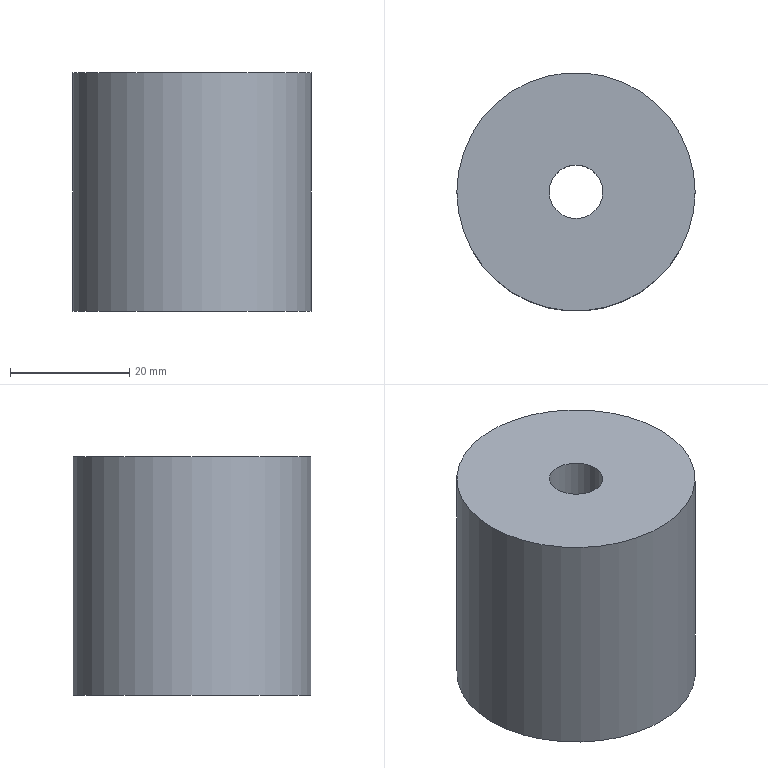Part | STEP file | gslz 2016.10.28-10_id2442_x_t | 1 solid | 6 faces | box 40 x 40 x 40 mm | volume 45553 mm3 | cylinder 3 | plane 3 | commonest cylinder face diameters 9 x1 14 x1 40 x1
STEP:
#1=CARTESIAN_POINT('',(0.,0.,0.));
#2=DIRECTION('',(0.,0.,1.));
#3=DIRECTION('',(1.,0.,0.));
#4=AXIS2_PLACEMENT_3D('',#1,#2,#3);
#5=CARTESIAN_POINT('',(-61.5,235.,105.));
#6=VERTEX_POINT('',#5);
#7=CARTESIAN_POINT('',(-81.5,235.,105.));
#8=DIRECTION('',(0.,0.,1.));
#9=DIRECTION('',(1.,0.,0.));
#10=AXIS2_PLACEMENT_3D('',#7,#8,#9);
#11=CIRCLE('',#10,20.);
#12=CARTESIAN_POINT('',(-81.5,235.,60.));
#13=DIRECTION('',(0.,0.,1.));
#14=DIRECTION('',(1.,0.,0.));
#15=AXIS2_PLACEMENT_3D('',#12,#13,#14);
#16=CYLINDRICAL_SURFACE('',#15,20.);
#17=CARTESIAN_POINT('',(0.,45.));
#18=DIRECTION('',(1.,0.));
#19=VECTOR('',#18,1.);
#20=LINE('',#17,#19);
#21=(GEOMETRIC_REPRESENTATION_CONTEXT(2)PARAMETRIC_REPRESENTATION_CONTEXT()REPRESENTATION_CONTEXT('',''));
#22=DEFINITIONAL_REPRESENTATION('',(#20),#21);
#23=PCURVE('',#16,#22);
#24=CARTESIAN_POINT('',(-29.389,-253.723,105.));
#25=DIRECTION('',(0.,0.,1.));
#26=DIRECTION('',(1.,0.,0.));
#27=AXIS2_PLACEMENT_3D('',#24,#25,#26);
#28=PLANE('',#27);
#29=CARTESIAN_POINT('',(-52.111,488.723));
#30=DIRECTION('',(1.,0.));
#31=AXIS2_PLACEMENT_2D('',#29,#30);
#32=CIRCLE('',#31,20.);
#33=(GEOMETRIC_REPRESENTATION_CONTEXT(2)PARAMETRIC_REPRESENTATION_CONTEXT()REPRESENTATION_CONTEXT('',''));
#34=DEFINITIONAL_REPRESENTATION('',(#32),#33);
#35=PCURVE('',#28,#34);
#36=SURFACE_CURVE('',#11,(#23,#35),.PCURVE_S1.);
#37=EDGE_CURVE('',#6,#6,#36,.T.);
#38=ORIENTED_EDGE('',*,*,#37,.F.);
#39=CARTESIAN_POINT('',(-61.5,235.,65.));
#40=VERTEX_POINT('',#39);
#41=CARTESIAN_POINT('',(-61.5,235.,65.));
#42=CARTESIAN_POINT('',(-61.5,235.,105.));
#43=B_SPLINE_CURVE_WITH_KNOTS('',1,(#41,#42),.UNSPECIFIED.,.F.,.F.,(2,2),(5.,45.),.PIECEWISE_BEZIER_KNOTS.);
#44=CARTESIAN_POINT('',(0.,0.));
#45=DIRECTION('',(0.,1.));
#46=VECTOR('',#45,1.);
#47=LINE('',#44,#46);
#48=(GEOMETRIC_REPRESENTATION_CONTEXT(2)PARAMETRIC_REPRESENTATION_CONTEXT()REPRESENTATION_CONTEXT('',''));
#49=DEFINITIONAL_REPRESENTATION('',(#47),#48);
#50=PCURVE('',#16,#49);
#51=CARTESIAN_POINT('',(6.283,0.));
#52=DIRECTION('',(0.,1.));
#53=VECTOR('',#52,1.);
#54=LINE('',#51,#53);
#55=(GEOMETRIC_REPRESENTATION_CONTEXT(2)PARAMETRIC_REPRESENTATION_CONTEXT()REPRESENTATION_CONTEXT('',''));
#56=DEFINITIONAL_REPRESENTATION('',(#54),#55);
#57=PCURVE('',#16,#56);
#58=SEAM_CURVE('',#43,(#50,#57),.PCURVE_S1.);
#59=EDGE_CURVE('',#40,#6,#58,.T.);
#60=ORIENTED_EDGE('',*,*,#59,.F.);
#61=CARTESIAN_POINT('',(-101.5,235.,65.));
#62=VERTEX_POINT('',#61);
#63=CARTESIAN_POINT('',(-81.5,235.,65.));
#64=DIRECTION('',(0.,0.,1.));
#65=DIRECTION('',(-1.,0.,0.));
#66=AXIS2_PLACEMENT_3D('',#63,#64,#65);
#67=CIRCLE('',#66,20.);
#68=CARTESIAN_POINT('',(-3.142,5.));
#69=DIRECTION('',(1.,0.));
#70=VECTOR('',#69,1.);
#71=LINE('',#68,#70);
#72=(GEOMETRIC_REPRESENTATION_CONTEXT(2)PARAMETRIC_REPRESENTATION_CONTEXT()REPRESENTATION_CONTEXT('',''));
#73=DEFINITIONAL_REPRESENTATION('',(#71),#72);
#74=PCURVE('',#16,#73);
#75=CARTESIAN_POINT('',(-81.5,235.,65.));
#76=DIRECTION('',(0.,0.,-1.));
#77=DIRECTION('',(-1.,0.,0.));
#78=AXIS2_PLACEMENT_3D('',#75,#76,#77);
#79=PLANE('',#78);
#80=CARTESIAN_POINT('',(20.,0.));
#81=CARTESIAN_POINT('',(20.,-34.641));
#82=CARTESIAN_POINT('',(-10.,-17.321));
#83=CARTESIAN_POINT('',(-40.,0.));
#84=CARTESIAN_POINT('',(-10.,17.321));
#85=CARTESIAN_POINT('',(20.,34.641));
#86=CARTESIAN_POINT('',(20.,0.));
#87=(BOUNDED_CURVE()B_SPLINE_CURVE(2,(#80,#81,#82,#83,#84,#85,#86),.UNSPECIFIED.,.T.,.F.)B_SPLINE_CURVE_WITH_KNOTS((1,2,2,2,2,1),(-2.094,0.,2.094,4.189,6.283,8.378),.UNSPECIFIED.)CURVE()GEOMETRIC_REPRESENTATION_ITEM()RATIONAL_B_SPLINE_CURVE((1.,0.5,1.,0.5,1.,0.5,1.))REPRESENTATION_ITEM(''));
#88=(GEOMETRIC_REPRESENTATION_CONTEXT(2)PARAMETRIC_REPRESENTATION_CONTEXT()REPRESENTATION_CONTEXT('',''));
#89=DEFINITIONAL_REPRESENTATION('',(#87),#88);
#90=PCURVE('',#79,#89);
#91=SURFACE_CURVE('',#67,(#74,#90),.PCURVE_S1.);
#92=EDGE_CURVE('',#40,#62,#91,.T.);
#93=ORIENTED_EDGE('',*,*,#92,.T.);
#94=CARTESIAN_POINT('',(-81.5,235.,65.));
#95=DIRECTION('',(0.,0.,1.));
#96=DIRECTION('',(-1.,0.,0.));
#97=AXIS2_PLACEMENT_3D('',#94,#95,#96);
#98=CIRCLE('',#97,20.);
#99=CARTESIAN_POINT('',(3.142,5.));
#100=DIRECTION('',(1.,0.));
#101=VECTOR('',#100,1.);
#102=LINE('',#99,#101);
#103=(GEOMETRIC_REPRESENTATION_CONTEXT(2)PARAMETRIC_REPRESENTATION_CONTEXT()REPRESENTATION_CONTEXT('',''));
#104=DEFINITIONAL_REPRESENTATION('',(#102),#103);
#105=PCURVE('',#16,#104);
#106=CARTESIAN_POINT('',(20.,0.));
#107=CARTESIAN_POINT('',(20.,-34.641));
#108=CARTESIAN_POINT('',(-10.,-17.321));
#109=CARTESIAN_POINT('',(-40.,0.));
#110=CARTESIAN_POINT('',(-10.,17.321));
#111=CARTESIAN_POINT('',(20.,34.641));
#112=CARTESIAN_POINT('',(20.,0.));
#113=(BOUNDED_CURVE()B_SPLINE_CURVE(2,(#106,#107,#108,#109,#110,#111,#112),.UNSPECIFIED.,.T.,.F.)B_SPLINE_CURVE_WITH_KNOTS((1,2,2,2,2,1),(-2.094,0.,2.094,4.189,6.283,8.378),.UNSPECIFIED.)CURVE()GEOMETRIC_REPRESENTATION_ITEM()RATIONAL_B_SPLINE_CURVE((1.,0.5,1.,0.5,1.,0.5,1.))REPRESENTATION_ITEM(''));
#114=(GEOMETRIC_REPRESENTATION_CONTEXT(2)PARAMETRIC_REPRESENTATION_CONTEXT()REPRESENTATION_CONTEXT('',''));
#115=DEFINITIONAL_REPRESENTATION('',(#113),#114);
#116=PCURVE('',#79,#115);
#117=SURFACE_CURVE('',#98,(#105,#116),.PCURVE_S1.);
#118=EDGE_CURVE('',#62,#40,#117,.T.);
#119=ORIENTED_EDGE('',*,*,#118,.T.);
#120=ORIENTED_EDGE('',*,*,#59,.T.);
#121=EDGE_LOOP('',(#38,#60,#93,#119,#120));
#122=FACE_BOUND('',#121,.T.);
#123=ADVANCED_FACE('',(#122),#16,.T.);
#124=CARTESIAN_POINT('',(-77.,235.,105.));
#125=VERTEX_POINT('',#124);
#126=CARTESIAN_POINT('',(-81.5,235.,105.));
#127=DIRECTION('',(0.,0.,1.));
#128=DIRECTION('',(1.,0.,0.));
#129=AXIS2_PLACEMENT_3D('',#126,#127,#128);
#130=CIRCLE('',#129,4.5);
#131=CARTESIAN_POINT('',(-52.111,488.723));
#132=DIRECTION('',(1.,0.));
#133=AXIS2_PLACEMENT_2D('',#131,#132);
#134=CIRCLE('',#133,4.5);
#135=(GEOMETRIC_REPRESENTATION_CONTEXT(2)PARAMETRIC_REPRESENTATION_CONTEXT()REPRESENTATION_CONTEXT('',''));
#136=DEFINITIONAL_REPRESENTATION('',(#134),#135);
#137=PCURVE('',#28,#136);
#138=CARTESIAN_POINT('',(-81.5,235.,37.));
#139=DIRECTION('',(0.,0.,1.));
#140=DIRECTION('',(1.,0.,0.));
#141=AXIS2_PLACEMENT_3D('',#138,#139,#140);
#142=CYLINDRICAL_SURFACE('',#141,4.5);
#143=CARTESIAN_POINT('',(0.,68.));
#144=DIRECTION('',(1.,0.));
#145=VECTOR('',#144,1.);
#146=LINE('',#143,#145);
#147=(GEOMETRIC_REPRESENTATION_CONTEXT(2)PARAMETRIC_REPRESENTATION_CONTEXT()REPRESENTATION_CONTEXT('',''));
#148=DEFINITIONAL_REPRESENTATION('',(#146),#147);
#149=PCURVE('',#142,#148);
#150=SURFACE_CURVE('',#130,(#137,#149),.PCURVE_S1.);
#151=EDGE_CURVE('',#125,#125,#150,.T.);
#152=ORIENTED_EDGE('',*,*,#151,.F.);
#153=EDGE_LOOP('',(#152));
#154=FACE_BOUND('',#153,.T.);
#155=ORIENTED_EDGE('',*,*,#37,.T.);
#156=EDGE_LOOP('',(#155));
#157=FACE_BOUND('',#156,.T.);
#158=ADVANCED_FACE('',(#154,#157),#28,.T.);
#159=ORIENTED_EDGE('',*,*,#118,.F.);
#160=ORIENTED_EDGE('',*,*,#92,.F.);
#161=EDGE_LOOP('',(#159,#160));
#162=FACE_BOUND('',#161,.T.);
#163=CARTESIAN_POINT('',(-88.5,235.,65.));
#164=VERTEX_POINT('',#163);
#165=CARTESIAN_POINT('',(-81.5,235.,65.));
#166=DIRECTION('',(0.,0.,1.));
#167=DIRECTION('',(-1.,0.,0.));
#168=AXIS2_PLACEMENT_3D('',#165,#166,#167);
#169=CIRCLE('',#168,7.);
#170=CARTESIAN_POINT('',(7.,0.));
#171=CARTESIAN_POINT('',(7.,-12.124));
#172=CARTESIAN_POINT('',(-3.5,-6.062));
#173=CARTESIAN_POINT('',(-14.,0.));
#174=CARTESIAN_POINT('',(-3.5,6.062));
#175=CARTESIAN_POINT('',(7.,12.124));
#176=CARTESIAN_POINT('',(7.,0.));
#177=(BOUNDED_CURVE()B_SPLINE_CURVE(2,(#170,#171,#172,#173,#174,#175,#176),.UNSPECIFIED.,.T.,.F.)B_SPLINE_CURVE_WITH_KNOTS((1,2,2,2,2,1),(-2.094,0.,2.094,4.189,6.283,8.378),.UNSPECIFIED.)CURVE()GEOMETRIC_REPRESENTATION_ITEM()RATIONAL_B_SPLINE_CURVE((1.,0.5,1.,0.5,1.,0.5,1.))REPRESENTATION_ITEM(''));
#178=(GEOMETRIC_REPRESENTATION_CONTEXT(2)PARAMETRIC_REPRESENTATION_CONTEXT()REPRESENTATION_CONTEXT('',''));
#179=DEFINITIONAL_REPRESENTATION('',(#177),#178);
#180=PCURVE('',#79,#179);
#181=CARTESIAN_POINT('',(-81.5,235.,65.));
#182=DIRECTION('',(0.,0.,1.));
#183=DIRECTION('',(1.,0.,0.));
#184=AXIS2_PLACEMENT_3D('',#181,#182,#183);
#185=CYLINDRICAL_SURFACE('',#184,7.);
#186=CARTESIAN_POINT('',(3.142,0.));
#187=DIRECTION('',(1.,0.));
#188=VECTOR('',#187,1.);
#189=LINE('',#186,#188);
#190=(GEOMETRIC_REPRESENTATION_CONTEXT(2)PARAMETRIC_REPRESENTATION_CONTEXT()REPRESENTATION_CONTEXT('',''));
#191=DEFINITIONAL_REPRESENTATION('',(#189),#190);
#192=PCURVE('',#185,#191);
#193=SURFACE_CURVE('',#169,(#180,#192),.PCURVE_S1.);
#194=EDGE_CURVE('',#164,#164,#193,.T.);
#195=ORIENTED_EDGE('',*,*,#194,.T.);
#196=EDGE_LOOP('',(#195));
#197=FACE_BOUND('',#196,.T.);
#198=ADVANCED_FACE('',(#162,#197),#79,.T.);
#199=ORIENTED_EDGE('',*,*,#151,.F.);
#200=CARTESIAN_POINT('',(-77.,235.,89.));
#201=VERTEX_POINT('',#200);
#202=CARTESIAN_POINT('',(-77.,235.,89.));
#203=CARTESIAN_POINT('',(-77.,235.,105.));
#204=B_SPLINE_CURVE_WITH_KNOTS('',1,(#202,#203),.UNSPECIFIED.,.F.,.F.,(2,2),(52.,68.),.PIECEWISE_BEZIER_KNOTS.);
#205=CARTESIAN_POINT('',(0.,0.));
#206=DIRECTION('',(0.,1.));
#207=VECTOR('',#206,1.);
#208=LINE('',#205,#207);
#209=(GEOMETRIC_REPRESENTATION_CONTEXT(2)PARAMETRIC_REPRESENTATION_CONTEXT()REPRESENTATION_CONTEXT('',''));
#210=DEFINITIONAL_REPRESENTATION('',(#208),#209);
#211=PCURVE('',#142,#210);
#212=CARTESIAN_POINT('',(6.283,0.));
#213=DIRECTION('',(0.,1.));
#214=VECTOR('',#213,1.);
#215=LINE('',#212,#214);
#216=(GEOMETRIC_REPRESENTATION_CONTEXT(2)PARAMETRIC_REPRESENTATION_CONTEXT()REPRESENTATION_CONTEXT('',''));
#217=DEFINITIONAL_REPRESENTATION('',(#215),#216);
#218=PCURVE('',#142,#217);
#219=SEAM_CURVE('',#204,(#211,#218),.PCURVE_S1.);
#220=EDGE_CURVE('',#201,#125,#219,.T.);
#221=ORIENTED_EDGE('',*,*,#220,.F.);
#222=CARTESIAN_POINT('',(-86.,235.,89.));
#223=VERTEX_POINT('',#222);
#224=CARTESIAN_POINT('',(-81.5,235.,89.));
#225=DIRECTION('',(0.,0.,-1.));
#226=DIRECTION('',(-1.,0.,0.));
#227=AXIS2_PLACEMENT_3D('',#224,#225,#226);
#228=CIRCLE('',#227,4.5);
#229=CARTESIAN_POINT('',(3.142,52.));
#230=DIRECTION('',(-1.,0.));
#231=VECTOR('',#230,1.);
#232=LINE('',#229,#231);
#233=(GEOMETRIC_REPRESENTATION_CONTEXT(2)PARAMETRIC_REPRESENTATION_CONTEXT()REPRESENTATION_CONTEXT('',''));
#234=DEFINITIONAL_REPRESENTATION('',(#232),#233);
#235=PCURVE('',#142,#234);
#236=CARTESIAN_POINT('',(-81.5,235.,89.));
#237=DIRECTION('',(0.,0.,-1.));
#238=DIRECTION('',(-1.,0.,0.));
#239=AXIS2_PLACEMENT_3D('',#236,#237,#238);
#240=PLANE('',#239);
#241=CARTESIAN_POINT('',(0.,0.));
#242=DIRECTION('',(1.,0.));
#243=AXIS2_PLACEMENT_2D('',#241,#242);
#244=CIRCLE('',#243,4.5);
#245=(GEOMETRIC_REPRESENTATION_CONTEXT(2)PARAMETRIC_REPRESENTATION_CONTEXT()REPRESENTATION_CONTEXT('',''));
#246=DEFINITIONAL_REPRESENTATION('',(#244),#245);
#247=PCURVE('',#240,#246);
#248=SURFACE_CURVE('',#228,(#235,#247),.PCURVE_S1.);
#249=EDGE_CURVE('',#223,#201,#248,.T.);
#250=ORIENTED_EDGE('',*,*,#249,.F.);
#251=CARTESIAN_POINT('',(-81.5,235.,89.));
#252=DIRECTION('',(0.,0.,-1.));
#253=DIRECTION('',(-1.,0.,0.));
#254=AXIS2_PLACEMENT_3D('',#251,#252,#253);
#255=CIRCLE('',#254,4.5);
#256=CARTESIAN_POINT('',(9.425,52.));
#257=DIRECTION('',(-1.,0.));
#258=VECTOR('',#257,1.);
#259=LINE('',#256,#258);
#260=(GEOMETRIC_REPRESENTATION_CONTEXT(2)PARAMETRIC_REPRESENTATION_CONTEXT()REPRESENTATION_CONTEXT('',''));
#261=DEFINITIONAL_REPRESENTATION('',(#259),#260);
#262=PCURVE('',#142,#261);
#263=CARTESIAN_POINT('',(0.,0.));
#264=DIRECTION('',(1.,0.));
#265=AXIS2_PLACEMENT_2D('',#263,#264);
#266=CIRCLE('',#265,4.5);
#267=(GEOMETRIC_REPRESENTATION_CONTEXT(2)PARAMETRIC_REPRESENTATION_CONTEXT()REPRESENTATION_CONTEXT('',''));
#268=DEFINITIONAL_REPRESENTATION('',(#266),#267);
#269=PCURVE('',#240,#268);
#270=SURFACE_CURVE('',#255,(#262,#269),.PCURVE_S1.);
#271=EDGE_CURVE('',#201,#223,#270,.T.);
#272=ORIENTED_EDGE('',*,*,#271,.F.);
#273=ORIENTED_EDGE('',*,*,#220,.T.);
#274=EDGE_LOOP('',(#199,#221,#250,#272,#273));
#275=FACE_BOUND('',#274,.F.);
#276=ADVANCED_FACE('',(#275),#142,.F.);
#277=CARTESIAN_POINT('',(-88.5,235.,89.));
#278=VERTEX_POINT('',#277);
#279=CARTESIAN_POINT('',(-81.5,235.,89.));
#280=DIRECTION('',(0.,0.,-1.));
#281=DIRECTION('',(-1.,0.,0.));
#282=AXIS2_PLACEMENT_3D('',#279,#280,#281);
#283=CIRCLE('',#282,7.);
#284=CARTESIAN_POINT('',(0.,0.));
#285=DIRECTION('',(1.,0.));
#286=AXIS2_PLACEMENT_2D('',#284,#285);
#287=CIRCLE('',#286,7.);
#288=(GEOMETRIC_REPRESENTATION_CONTEXT(2)PARAMETRIC_REPRESENTATION_CONTEXT()REPRESENTATION_CONTEXT('',''));
#289=DEFINITIONAL_REPRESENTATION('',(#287),#288);
#290=PCURVE('',#240,#289);
#291=CARTESIAN_POINT('',(9.425,24.));
#292=DIRECTION('',(-1.,0.));
#293=VECTOR('',#292,1.);
#294=LINE('',#291,#293);
#295=(GEOMETRIC_REPRESENTATION_CONTEXT(2)PARAMETRIC_REPRESENTATION_CONTEXT()REPRESENTATION_CONTEXT('',''));
#296=DEFINITIONAL_REPRESENTATION('',(#294),#295);
#297=PCURVE('',#185,#296);
#298=SURFACE_CURVE('',#283,(#290,#297),.PCURVE_S1.);
#299=EDGE_CURVE('',#278,#278,#298,.T.);
#300=ORIENTED_EDGE('',*,*,#299,.T.);
#301=EDGE_LOOP('',(#300));
#302=FACE_BOUND('',#301,.T.);
#303=ORIENTED_EDGE('',*,*,#249,.F.);
#304=ORIENTED_EDGE('',*,*,#271,.F.);
#305=EDGE_LOOP('',(#303,#304));
#306=FACE_BOUND('',#305,.T.);
#307=ADVANCED_FACE('',(#302,#306),#240,.T.);
#308=ORIENTED_EDGE('',*,*,#194,.T.);
#309=CARTESIAN_POINT('',(-88.5,235.,65.));
#310=CARTESIAN_POINT('',(-88.5,235.,89.));
#311=B_SPLINE_CURVE_WITH_KNOTS('',1,(#309,#310),.UNSPECIFIED.,.F.,.F.,(2,2),(0.,24.),.PIECEWISE_BEZIER_KNOTS.);
#312=CARTESIAN_POINT('',(9.425,0.));
#313=DIRECTION('',(0.,1.));
#314=VECTOR('',#313,1.);
#315=LINE('',#312,#314);
#316=(GEOMETRIC_REPRESENTATION_CONTEXT(2)PARAMETRIC_REPRESENTATION_CONTEXT()REPRESENTATION_CONTEXT('',''));
#317=DEFINITIONAL_REPRESENTATION('',(#315),#316);
#318=PCURVE('',#185,#317);
#319=CARTESIAN_POINT('',(3.142,0.));
#320=DIRECTION('',(0.,1.));
#321=VECTOR('',#320,1.);
#322=LINE('',#319,#321);
#323=(GEOMETRIC_REPRESENTATION_CONTEXT(2)PARAMETRIC_REPRESENTATION_CONTEXT()REPRESENTATION_CONTEXT('',''));
#324=DEFINITIONAL_REPRESENTATION('',(#322),#323);
#325=PCURVE('',#185,#324);
#326=SEAM_CURVE('',#311,(#318,#325),.PCURVE_S1.);
#327=EDGE_CURVE('',#164,#278,#326,.T.);
#328=ORIENTED_EDGE('',*,*,#327,.T.);
#329=ORIENTED_EDGE('',*,*,#299,.T.);
#330=ORIENTED_EDGE('',*,*,#327,.F.);
#331=EDGE_LOOP('',(#308,#328,#329,#330));
#332=FACE_BOUND('',#331,.F.);
#333=ADVANCED_FACE('',(#332),#185,.F.);
#334=CLOSED_SHELL('',(#123,#158,#198,#276,#307,#333));
#335=MANIFOLD_SOLID_BREP('',#334);
#336=(LENGTH_UNIT()NAMED_UNIT(*)SI_UNIT(.MILLI.,.METRE.));
#337=UNCERTAINTY_MEASURE_WITH_UNIT(LENGTH_MEASURE(0.000005),#336,'','');
#338=(NAMED_UNIT(*)PLANE_ANGLE_UNIT()SI_UNIT($,.RADIAN.));
#339=(NAMED_UNIT(*)SI_UNIT($,.STERADIAN.)SOLID_ANGLE_UNIT());
#340=(GEOMETRIC_REPRESENTATION_CONTEXT(3)GLOBAL_UNCERTAINTY_ASSIGNED_CONTEXT((#337))GLOBAL_UNIT_ASSIGNED_CONTEXT((#336,#338,#339))REPRESENTATION_CONTEXT('',''));
#341=ADVANCED_BREP_SHAPE_REPRESENTATION('',(#4,#335),#340);